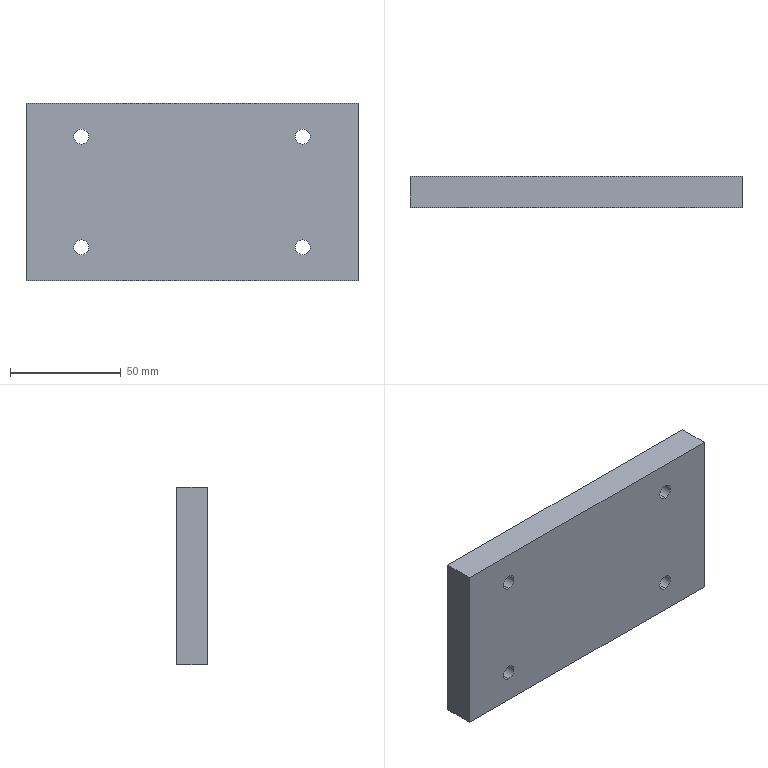Part | SolidWorks | features Extrusion 1, HoleWzd 1 | 1 solid | 14 faces | box 150 x 14 x 80 mm | volume 165966 mm3 | cylinder 8 | plane 6 | commonest cylinder face diameters 6.8 x8
STEP:
#1=CARTESIAN_POINT('',(25.,0.,-68.4));
#2=VERTEX_POINT('',#1);
#3=CARTESIAN_POINT('',(25.,0.,-61.6));
#4=VERTEX_POINT('',#3);
#5=CARTESIAN_POINT('',(25.,0.,-65.));
#6=DIRECTION('',(0.,1.,0.));
#7=DIRECTION('',(0.,0.,1.));
#8=AXIS2_PLACEMENT_3D('',#5,#6,#7);
#9=CIRCLE('',#8,3.4);
#10=EDGE_CURVE('',#2,#4,#9,.T.);
#11=ORIENTED_EDGE('',*,*,#10,.F.);
#12=CARTESIAN_POINT('',(25.,14.,-68.4));
#13=VERTEX_POINT('',#12);
#14=CARTESIAN_POINT('',(25.,14.,-68.4));
#15=DIRECTION('',(0.,1.,0.));
#16=VECTOR('',#15,1000.);
#17=LINE('',#14,#16);
#18=EDGE_CURVE('',#2,#13,#17,.T.);
#19=ORIENTED_EDGE('',*,*,#18,.T.);
#20=CARTESIAN_POINT('',(25.,14.,-61.6));
#21=VERTEX_POINT('',#20);
#22=CARTESIAN_POINT('',(25.,14.,-65.));
#23=DIRECTION('',(0.,1.,0.));
#24=DIRECTION('',(0.,0.,1.));
#25=AXIS2_PLACEMENT_3D('',#22,#23,#24);
#26=CIRCLE('',#25,3.4);
#27=EDGE_CURVE('',#13,#21,#26,.T.);
#28=ORIENTED_EDGE('',*,*,#27,.T.);
#29=CARTESIAN_POINT('',(25.,14.,-61.6));
#30=DIRECTION('',(0.,1.,0.));
#31=VECTOR('',#30,1000.);
#32=LINE('',#29,#31);
#33=EDGE_CURVE('',#4,#21,#32,.T.);
#34=ORIENTED_EDGE('',*,*,#33,.F.);
#35=EDGE_LOOP('',(#11,#19,#28,#34));
#36=FACE_OUTER_BOUND('',#35,.T.);
#37=CARTESIAN_POINT('',(25.,14.,-65.));
#38=DIRECTION('',(0.,1.,0.));
#39=DIRECTION('',(0.,0.,1.));
#40=AXIS2_PLACEMENT_3D('',#37,#38,#39);
#41=CYLINDRICAL_SURFACE('',#40,3.4);
#42=ADVANCED_FACE('',(#36),#41,.F.);
#43=CARTESIAN_POINT('',(25.,0.,-18.4));
#44=VERTEX_POINT('',#43);
#45=CARTESIAN_POINT('',(25.,0.,-11.6));
#46=VERTEX_POINT('',#45);
#47=CARTESIAN_POINT('',(25.,0.,-15.));
#48=DIRECTION('',(0.,1.,0.));
#49=DIRECTION('',(0.,0.,1.));
#50=AXIS2_PLACEMENT_3D('',#47,#48,#49);
#51=CIRCLE('',#50,3.4);
#52=EDGE_CURVE('',#44,#46,#51,.T.);
#53=ORIENTED_EDGE('',*,*,#52,.F.);
#54=CARTESIAN_POINT('',(25.,14.,-18.4));
#55=VERTEX_POINT('',#54);
#56=CARTESIAN_POINT('',(25.,14.,-18.4));
#57=DIRECTION('',(0.,1.,0.));
#58=VECTOR('',#57,1000.);
#59=LINE('',#56,#58);
#60=EDGE_CURVE('',#44,#55,#59,.T.);
#61=ORIENTED_EDGE('',*,*,#60,.T.);
#62=CARTESIAN_POINT('',(25.,14.,-11.6));
#63=VERTEX_POINT('',#62);
#64=CARTESIAN_POINT('',(25.,14.,-15.));
#65=DIRECTION('',(0.,1.,0.));
#66=DIRECTION('',(0.,0.,1.));
#67=AXIS2_PLACEMENT_3D('',#64,#65,#66);
#68=CIRCLE('',#67,3.4);
#69=EDGE_CURVE('',#55,#63,#68,.T.);
#70=ORIENTED_EDGE('',*,*,#69,.T.);
#71=CARTESIAN_POINT('',(25.,14.,-11.6));
#72=DIRECTION('',(0.,1.,0.));
#73=VECTOR('',#72,1000.);
#74=LINE('',#71,#73);
#75=EDGE_CURVE('',#46,#63,#74,.T.);
#76=ORIENTED_EDGE('',*,*,#75,.F.);
#77=EDGE_LOOP('',(#53,#61,#70,#76));
#78=FACE_OUTER_BOUND('',#77,.T.);
#79=CARTESIAN_POINT('',(25.,14.,-15.));
#80=DIRECTION('',(0.,1.,0.));
#81=DIRECTION('',(0.,0.,1.));
#82=AXIS2_PLACEMENT_3D('',#79,#80,#81);
#83=CYLINDRICAL_SURFACE('',#82,3.4);
#84=ADVANCED_FACE('',(#78),#83,.F.);
#85=CARTESIAN_POINT('',(125.,0.,-18.4));
#86=VERTEX_POINT('',#85);
#87=CARTESIAN_POINT('',(125.,0.,-11.6));
#88=VERTEX_POINT('',#87);
#89=CARTESIAN_POINT('',(125.,0.,-15.));
#90=DIRECTION('',(0.,1.,0.));
#91=DIRECTION('',(0.,0.,1.));
#92=AXIS2_PLACEMENT_3D('',#89,#90,#91);
#93=CIRCLE('',#92,3.4);
#94=EDGE_CURVE('',#86,#88,#93,.T.);
#95=ORIENTED_EDGE('',*,*,#94,.F.);
#96=CARTESIAN_POINT('',(125.,14.,-18.4));
#97=VERTEX_POINT('',#96);
#98=CARTESIAN_POINT('',(125.,14.,-18.4));
#99=DIRECTION('',(0.,1.,0.));
#100=VECTOR('',#99,1000.);
#101=LINE('',#98,#100);
#102=EDGE_CURVE('',#86,#97,#101,.T.);
#103=ORIENTED_EDGE('',*,*,#102,.T.);
#104=CARTESIAN_POINT('',(125.,14.,-11.6));
#105=VERTEX_POINT('',#104);
#106=CARTESIAN_POINT('',(125.,14.,-15.));
#107=DIRECTION('',(0.,1.,0.));
#108=DIRECTION('',(0.,0.,1.));
#109=AXIS2_PLACEMENT_3D('',#106,#107,#108);
#110=CIRCLE('',#109,3.4);
#111=EDGE_CURVE('',#97,#105,#110,.T.);
#112=ORIENTED_EDGE('',*,*,#111,.T.);
#113=CARTESIAN_POINT('',(125.,14.,-11.6));
#114=DIRECTION('',(0.,1.,0.));
#115=VECTOR('',#114,1000.);
#116=LINE('',#113,#115);
#117=EDGE_CURVE('',#88,#105,#116,.T.);
#118=ORIENTED_EDGE('',*,*,#117,.F.);
#119=EDGE_LOOP('',(#95,#103,#112,#118));
#120=FACE_OUTER_BOUND('',#119,.T.);
#121=CARTESIAN_POINT('',(125.,14.,-15.));
#122=DIRECTION('',(0.,1.,0.));
#123=DIRECTION('',(0.,0.,1.));
#124=AXIS2_PLACEMENT_3D('',#121,#122,#123);
#125=CYLINDRICAL_SURFACE('',#124,3.4);
#126=ADVANCED_FACE('',(#120),#125,.F.);
#127=CARTESIAN_POINT('',(125.,0.,-68.4));
#128=VERTEX_POINT('',#127);
#129=CARTESIAN_POINT('',(125.,0.,-61.6));
#130=VERTEX_POINT('',#129);
#131=CARTESIAN_POINT('',(125.,0.,-65.));
#132=DIRECTION('',(0.,1.,0.));
#133=DIRECTION('',(0.,0.,1.));
#134=AXIS2_PLACEMENT_3D('',#131,#132,#133);
#135=CIRCLE('',#134,3.4);
#136=EDGE_CURVE('',#128,#130,#135,.T.);
#137=ORIENTED_EDGE('',*,*,#136,.F.);
#138=CARTESIAN_POINT('',(125.,14.,-68.4));
#139=VERTEX_POINT('',#138);
#140=CARTESIAN_POINT('',(125.,14.,-68.4));
#141=DIRECTION('',(0.,1.,0.));
#142=VECTOR('',#141,1000.);
#143=LINE('',#140,#142);
#144=EDGE_CURVE('',#128,#139,#143,.T.);
#145=ORIENTED_EDGE('',*,*,#144,.T.);
#146=CARTESIAN_POINT('',(125.,14.,-61.6));
#147=VERTEX_POINT('',#146);
#148=CARTESIAN_POINT('',(125.,14.,-65.));
#149=DIRECTION('',(0.,1.,0.));
#150=DIRECTION('',(0.,0.,1.));
#151=AXIS2_PLACEMENT_3D('',#148,#149,#150);
#152=CIRCLE('',#151,3.4);
#153=EDGE_CURVE('',#139,#147,#152,.T.);
#154=ORIENTED_EDGE('',*,*,#153,.T.);
#155=CARTESIAN_POINT('',(125.,14.,-61.6));
#156=DIRECTION('',(0.,1.,0.));
#157=VECTOR('',#156,1000.);
#158=LINE('',#155,#157);
#159=EDGE_CURVE('',#130,#147,#158,.T.);
#160=ORIENTED_EDGE('',*,*,#159,.F.);
#161=EDGE_LOOP('',(#137,#145,#154,#160));
#162=FACE_OUTER_BOUND('',#161,.T.);
#163=CARTESIAN_POINT('',(125.,14.,-65.));
#164=DIRECTION('',(0.,1.,0.));
#165=DIRECTION('',(0.,0.,1.));
#166=AXIS2_PLACEMENT_3D('',#163,#164,#165);
#167=CYLINDRICAL_SURFACE('',#166,3.4);
#168=ADVANCED_FACE('',(#162),#167,.F.);
#169=CARTESIAN_POINT('',(0.,0.,-80.));
#170=VERTEX_POINT('',#169);
#171=CARTESIAN_POINT('',(0.,0.,0.));
#172=VERTEX_POINT('',#171);
#173=CARTESIAN_POINT('',(0.,0.,0.));
#174=DIRECTION('',(0.,0.,1.));
#175=VECTOR('',#174,1000.);
#176=LINE('',#173,#175);
#177=EDGE_CURVE('',#170,#172,#176,.T.);
#178=ORIENTED_EDGE('',*,*,#177,.T.);
#179=CARTESIAN_POINT('',(0.,14.,0.));
#180=VERTEX_POINT('',#179);
#181=CARTESIAN_POINT('',(0.,14.,0.));
#182=DIRECTION('',(0.,-1.,0.));
#183=VECTOR('',#182,1000.);
#184=LINE('',#181,#183);
#185=EDGE_CURVE('',#180,#172,#184,.T.);
#186=ORIENTED_EDGE('',*,*,#185,.F.);
#187=CARTESIAN_POINT('',(0.,14.,-80.));
#188=VERTEX_POINT('',#187);
#189=CARTESIAN_POINT('',(0.,14.,0.));
#190=DIRECTION('',(0.,0.,1.));
#191=VECTOR('',#190,1000.);
#192=LINE('',#189,#191);
#193=EDGE_CURVE('',#188,#180,#192,.T.);
#194=ORIENTED_EDGE('',*,*,#193,.F.);
#195=CARTESIAN_POINT('',(0.,14.,-80.));
#196=DIRECTION('',(0.,-1.,0.));
#197=VECTOR('',#196,1000.);
#198=LINE('',#195,#197);
#199=EDGE_CURVE('',#188,#170,#198,.T.);
#200=ORIENTED_EDGE('',*,*,#199,.T.);
#201=EDGE_LOOP('',(#178,#186,#194,#200));
#202=FACE_OUTER_BOUND('',#201,.T.);
#203=CARTESIAN_POINT('',(0.,14.,0.));
#204=DIRECTION('',(1.,0.,0.));
#205=DIRECTION('',(0.,0.,-1.));
#206=AXIS2_PLACEMENT_3D('',#203,#204,#205);
#207=PLANE('',#206);
#208=ADVANCED_FACE('',(#202),#207,.F.);
#209=CARTESIAN_POINT('',(150.,0.,0.));
#210=VERTEX_POINT('',#209);
#211=CARTESIAN_POINT('',(0.,0.,0.));
#212=DIRECTION('',(1.,0.,0.));
#213=VECTOR('',#212,1000.);
#214=LINE('',#211,#213);
#215=EDGE_CURVE('',#172,#210,#214,.T.);
#216=ORIENTED_EDGE('',*,*,#215,.T.);
#217=CARTESIAN_POINT('',(150.,14.,0.));
#218=VERTEX_POINT('',#217);
#219=CARTESIAN_POINT('',(150.,14.,0.));
#220=DIRECTION('',(0.,-1.,0.));
#221=VECTOR('',#220,1000.);
#222=LINE('',#219,#221);
#223=EDGE_CURVE('',#218,#210,#222,.T.);
#224=ORIENTED_EDGE('',*,*,#223,.F.);
#225=CARTESIAN_POINT('',(0.,14.,0.));
#226=DIRECTION('',(1.,0.,0.));
#227=VECTOR('',#226,1000.);
#228=LINE('',#225,#227);
#229=EDGE_CURVE('',#180,#218,#228,.T.);
#230=ORIENTED_EDGE('',*,*,#229,.F.);
#231=ORIENTED_EDGE('',*,*,#185,.T.);
#232=EDGE_LOOP('',(#216,#224,#230,#231));
#233=FACE_OUTER_BOUND('',#232,.T.);
#234=CARTESIAN_POINT('',(0.,14.,0.));
#235=DIRECTION('',(0.,0.,-1.));
#236=DIRECTION('',(-1.,0.,0.));
#237=AXIS2_PLACEMENT_3D('',#234,#235,#236);
#238=PLANE('',#237);
#239=ADVANCED_FACE('',(#233),#238,.F.);
#240=CARTESIAN_POINT('',(150.,0.,-80.));
#241=VERTEX_POINT('',#240);
#242=CARTESIAN_POINT('',(150.,0.,0.));
#243=DIRECTION('',(0.,0.,-1.));
#244=VECTOR('',#243,1000.);
#245=LINE('',#242,#244);
#246=EDGE_CURVE('',#210,#241,#245,.T.);
#247=ORIENTED_EDGE('',*,*,#246,.T.);
#248=CARTESIAN_POINT('',(150.,14.,-80.));
#249=VERTEX_POINT('',#248);
#250=CARTESIAN_POINT('',(150.,14.,-80.));
#251=DIRECTION('',(0.,-1.,0.));
#252=VECTOR('',#251,1000.);
#253=LINE('',#250,#252);
#254=EDGE_CURVE('',#249,#241,#253,.T.);
#255=ORIENTED_EDGE('',*,*,#254,.F.);
#256=CARTESIAN_POINT('',(150.,14.,0.));
#257=DIRECTION('',(0.,0.,-1.));
#258=VECTOR('',#257,1000.);
#259=LINE('',#256,#258);
#260=EDGE_CURVE('',#218,#249,#259,.T.);
#261=ORIENTED_EDGE('',*,*,#260,.F.);
#262=ORIENTED_EDGE('',*,*,#223,.T.);
#263=EDGE_LOOP('',(#247,#255,#261,#262));
#264=FACE_OUTER_BOUND('',#263,.T.);
#265=CARTESIAN_POINT('',(150.,14.,0.));
#266=DIRECTION('',(-1.,0.,0.));
#267=DIRECTION('',(0.,0.,1.));
#268=AXIS2_PLACEMENT_3D('',#265,#266,#267);
#269=PLANE('',#268);
#270=ADVANCED_FACE('',(#264),#269,.F.);
#271=CARTESIAN_POINT('',(0.,0.,-80.));
#272=DIRECTION('',(-1.,0.,0.));
#273=VECTOR('',#272,1000.);
#274=LINE('',#271,#273);
#275=EDGE_CURVE('',#241,#170,#274,.T.);
#276=ORIENTED_EDGE('',*,*,#275,.T.);
#277=ORIENTED_EDGE('',*,*,#199,.F.);
#278=CARTESIAN_POINT('',(0.,14.,-80.));
#279=DIRECTION('',(-1.,0.,0.));
#280=VECTOR('',#279,1000.);
#281=LINE('',#278,#280);
#282=EDGE_CURVE('',#249,#188,#281,.T.);
#283=ORIENTED_EDGE('',*,*,#282,.F.);
#284=ORIENTED_EDGE('',*,*,#254,.T.);
#285=EDGE_LOOP('',(#276,#277,#283,#284));
#286=FACE_OUTER_BOUND('',#285,.T.);
#287=CARTESIAN_POINT('',(0.,14.,-80.));
#288=DIRECTION('',(0.,0.,1.));
#289=DIRECTION('',(1.,0.,0.));
#290=AXIS2_PLACEMENT_3D('',#287,#288,#289);
#291=PLANE('',#290);
#292=ADVANCED_FACE('',(#286),#291,.F.);
#293=CARTESIAN_POINT('',(25.,14.,-65.));
#294=DIRECTION('',(0.,1.,0.));
#295=DIRECTION('',(0.,0.,1.));
#296=AXIS2_PLACEMENT_3D('',#293,#294,#295);
#297=CIRCLE('',#296,3.4);
#298=EDGE_CURVE('',#21,#13,#297,.T.);
#299=ORIENTED_EDGE('',*,*,#298,.F.);
#300=ORIENTED_EDGE('',*,*,#27,.F.);
#301=EDGE_LOOP('',(#299,#300));
#302=FACE_BOUND('',#301,.T.);
#303=CARTESIAN_POINT('',(25.,14.,-15.));
#304=DIRECTION('',(0.,1.,0.));
#305=DIRECTION('',(0.,0.,1.));
#306=AXIS2_PLACEMENT_3D('',#303,#304,#305);
#307=CIRCLE('',#306,3.4);
#308=EDGE_CURVE('',#63,#55,#307,.T.);
#309=ORIENTED_EDGE('',*,*,#308,.F.);
#310=ORIENTED_EDGE('',*,*,#69,.F.);
#311=EDGE_LOOP('',(#309,#310));
#312=FACE_BOUND('',#311,.T.);
#313=CARTESIAN_POINT('',(125.,14.,-15.));
#314=DIRECTION('',(0.,1.,0.));
#315=DIRECTION('',(0.,0.,1.));
#316=AXIS2_PLACEMENT_3D('',#313,#314,#315);
#317=CIRCLE('',#316,3.4);
#318=EDGE_CURVE('',#105,#97,#317,.T.);
#319=ORIENTED_EDGE('',*,*,#318,.F.);
#320=ORIENTED_EDGE('',*,*,#111,.F.);
#321=EDGE_LOOP('',(#319,#320));
#322=FACE_BOUND('',#321,.T.);
#323=CARTESIAN_POINT('',(125.,14.,-65.));
#324=DIRECTION('',(0.,1.,0.));
#325=DIRECTION('',(0.,0.,1.));
#326=AXIS2_PLACEMENT_3D('',#323,#324,#325);
#327=CIRCLE('',#326,3.4);
#328=EDGE_CURVE('',#147,#139,#327,.T.);
#329=ORIENTED_EDGE('',*,*,#328,.F.);
#330=ORIENTED_EDGE('',*,*,#153,.F.);
#331=EDGE_LOOP('',(#329,#330));
#332=FACE_BOUND('',#331,.T.);
#333=ORIENTED_EDGE('',*,*,#193,.T.);
#334=ORIENTED_EDGE('',*,*,#229,.T.);
#335=ORIENTED_EDGE('',*,*,#260,.T.);
#336=ORIENTED_EDGE('',*,*,#282,.T.);
#337=EDGE_LOOP('',(#333,#334,#335,#336));
#338=FACE_OUTER_BOUND('',#337,.T.);
#339=CARTESIAN_POINT('',(0.,14.,0.));
#340=DIRECTION('',(0.,-1.,0.));
#341=DIRECTION('',(0.,0.,-1.));
#342=AXIS2_PLACEMENT_3D('',#339,#340,#341);
#343=PLANE('',#342);
#344=ADVANCED_FACE('',(#302,#312,#322,#332,#338),#343,.F.);
#345=CARTESIAN_POINT('',(25.,0.,-65.));
#346=DIRECTION('',(0.,1.,0.));
#347=DIRECTION('',(0.,0.,1.));
#348=AXIS2_PLACEMENT_3D('',#345,#346,#347);
#349=CIRCLE('',#348,3.4);
#350=EDGE_CURVE('',#4,#2,#349,.T.);
#351=ORIENTED_EDGE('',*,*,#350,.T.);
#352=ORIENTED_EDGE('',*,*,#10,.T.);
#353=EDGE_LOOP('',(#351,#352));
#354=FACE_BOUND('',#353,.T.);
#355=CARTESIAN_POINT('',(25.,0.,-15.));
#356=DIRECTION('',(0.,1.,0.));
#357=DIRECTION('',(0.,0.,1.));
#358=AXIS2_PLACEMENT_3D('',#355,#356,#357);
#359=CIRCLE('',#358,3.4);
#360=EDGE_CURVE('',#46,#44,#359,.T.);
#361=ORIENTED_EDGE('',*,*,#360,.T.);
#362=ORIENTED_EDGE('',*,*,#52,.T.);
#363=EDGE_LOOP('',(#361,#362));
#364=FACE_BOUND('',#363,.T.);
#365=CARTESIAN_POINT('',(125.,0.,-15.));
#366=DIRECTION('',(0.,1.,0.));
#367=DIRECTION('',(0.,0.,1.));
#368=AXIS2_PLACEMENT_3D('',#365,#366,#367);
#369=CIRCLE('',#368,3.4);
#370=EDGE_CURVE('',#88,#86,#369,.T.);
#371=ORIENTED_EDGE('',*,*,#370,.T.);
#372=ORIENTED_EDGE('',*,*,#94,.T.);
#373=EDGE_LOOP('',(#371,#372));
#374=FACE_BOUND('',#373,.T.);
#375=CARTESIAN_POINT('',(125.,0.,-65.));
#376=DIRECTION('',(0.,1.,0.));
#377=DIRECTION('',(0.,0.,1.));
#378=AXIS2_PLACEMENT_3D('',#375,#376,#377);
#379=CIRCLE('',#378,3.4);
#380=EDGE_CURVE('',#130,#128,#379,.T.);
#381=ORIENTED_EDGE('',*,*,#380,.T.);
#382=ORIENTED_EDGE('',*,*,#136,.T.);
#383=EDGE_LOOP('',(#381,#382));
#384=FACE_BOUND('',#383,.T.);
#385=ORIENTED_EDGE('',*,*,#177,.F.);
#386=ORIENTED_EDGE('',*,*,#275,.F.);
#387=ORIENTED_EDGE('',*,*,#246,.F.);
#388=ORIENTED_EDGE('',*,*,#215,.F.);
#389=EDGE_LOOP('',(#385,#386,#387,#388));
#390=FACE_OUTER_BOUND('',#389,.T.);
#391=CARTESIAN_POINT('',(0.,0.,0.));
#392=DIRECTION('',(0.,-1.,0.));
#393=DIRECTION('',(0.,0.,-1.));
#394=AXIS2_PLACEMENT_3D('',#391,#392,#393);
#395=PLANE('',#394);
#396=ADVANCED_FACE('',(#354,#364,#374,#384,#390),#395,.T.);
#397=ORIENTED_EDGE('',*,*,#144,.F.);
#398=ORIENTED_EDGE('',*,*,#380,.F.);
#399=ORIENTED_EDGE('',*,*,#159,.T.);
#400=ORIENTED_EDGE('',*,*,#328,.T.);
#401=EDGE_LOOP('',(#397,#398,#399,#400));
#402=FACE_OUTER_BOUND('',#401,.T.);
#403=CARTESIAN_POINT('',(125.,14.,-65.));
#404=DIRECTION('',(0.,1.,0.));
#405=DIRECTION('',(0.,0.,1.));
#406=AXIS2_PLACEMENT_3D('',#403,#404,#405);
#407=CYLINDRICAL_SURFACE('',#406,3.4);
#408=ADVANCED_FACE('',(#402),#407,.F.);
#409=ORIENTED_EDGE('',*,*,#102,.F.);
#410=ORIENTED_EDGE('',*,*,#370,.F.);
#411=ORIENTED_EDGE('',*,*,#117,.T.);
#412=ORIENTED_EDGE('',*,*,#318,.T.);
#413=EDGE_LOOP('',(#409,#410,#411,#412));
#414=FACE_OUTER_BOUND('',#413,.T.);
#415=CARTESIAN_POINT('',(125.,14.,-15.));
#416=DIRECTION('',(0.,1.,0.));
#417=DIRECTION('',(0.,0.,1.));
#418=AXIS2_PLACEMENT_3D('',#415,#416,#417);
#419=CYLINDRICAL_SURFACE('',#418,3.4);
#420=ADVANCED_FACE('',(#414),#419,.F.);
#421=ORIENTED_EDGE('',*,*,#60,.F.);
#422=ORIENTED_EDGE('',*,*,#360,.F.);
#423=ORIENTED_EDGE('',*,*,#75,.T.);
#424=ORIENTED_EDGE('',*,*,#308,.T.);
#425=EDGE_LOOP('',(#421,#422,#423,#424));
#426=FACE_OUTER_BOUND('',#425,.T.);
#427=CARTESIAN_POINT('',(25.,14.,-15.));
#428=DIRECTION('',(0.,1.,0.));
#429=DIRECTION('',(0.,0.,1.));
#430=AXIS2_PLACEMENT_3D('',#427,#428,#429);
#431=CYLINDRICAL_SURFACE('',#430,3.4);
#432=ADVANCED_FACE('',(#426),#431,.F.);
#433=ORIENTED_EDGE('',*,*,#18,.F.);
#434=ORIENTED_EDGE('',*,*,#350,.F.);
#435=ORIENTED_EDGE('',*,*,#33,.T.);
#436=ORIENTED_EDGE('',*,*,#298,.T.);
#437=EDGE_LOOP('',(#433,#434,#435,#436));
#438=FACE_OUTER_BOUND('',#437,.T.);
#439=CARTESIAN_POINT('',(25.,14.,-65.));
#440=DIRECTION('',(0.,1.,0.));
#441=DIRECTION('',(0.,0.,1.));
#442=AXIS2_PLACEMENT_3D('',#439,#440,#441);
#443=CYLINDRICAL_SURFACE('',#442,3.4);
#444=ADVANCED_FACE('',(#438),#443,.F.);
#445=CLOSED_SHELL('',(#42,#84,#126,#168,#208,#239,#270,#292,#344,#396,#408,#420,#432,#444));
#446=MANIFOLD_SOLID_BREP('',#445);
#447=CARTESIAN_POINT('',(0.,0.,0.));
#448=DIRECTION('',(0.,0.,1.));
#449=DIRECTION('',(1.,0.,0.));
#450=AXIS2_PLACEMENT_3D('',#447,#448,#449);
#451=(LENGTH_UNIT()NAMED_UNIT(*)SI_UNIT(.MILLI.,.METRE.));
#452=UNCERTAINTY_MEASURE_WITH_UNIT(LENGTH_MEASURE(0.00001),#451,'','');
#453=(NAMED_UNIT(*)PLANE_ANGLE_UNIT()SI_UNIT($,.RADIAN.));
#454=(NAMED_UNIT(*)SI_UNIT($,.STERADIAN.)SOLID_ANGLE_UNIT());
#455=(GEOMETRIC_REPRESENTATION_CONTEXT(3)GLOBAL_UNCERTAINTY_ASSIGNED_CONTEXT((#452))GLOBAL_UNIT_ASSIGNED_CONTEXT((#451,#453,#454))REPRESENTATION_CONTEXT('',''));
#456=ADVANCED_BREP_SHAPE_REPRESENTATION('',(#446,#450),#455);